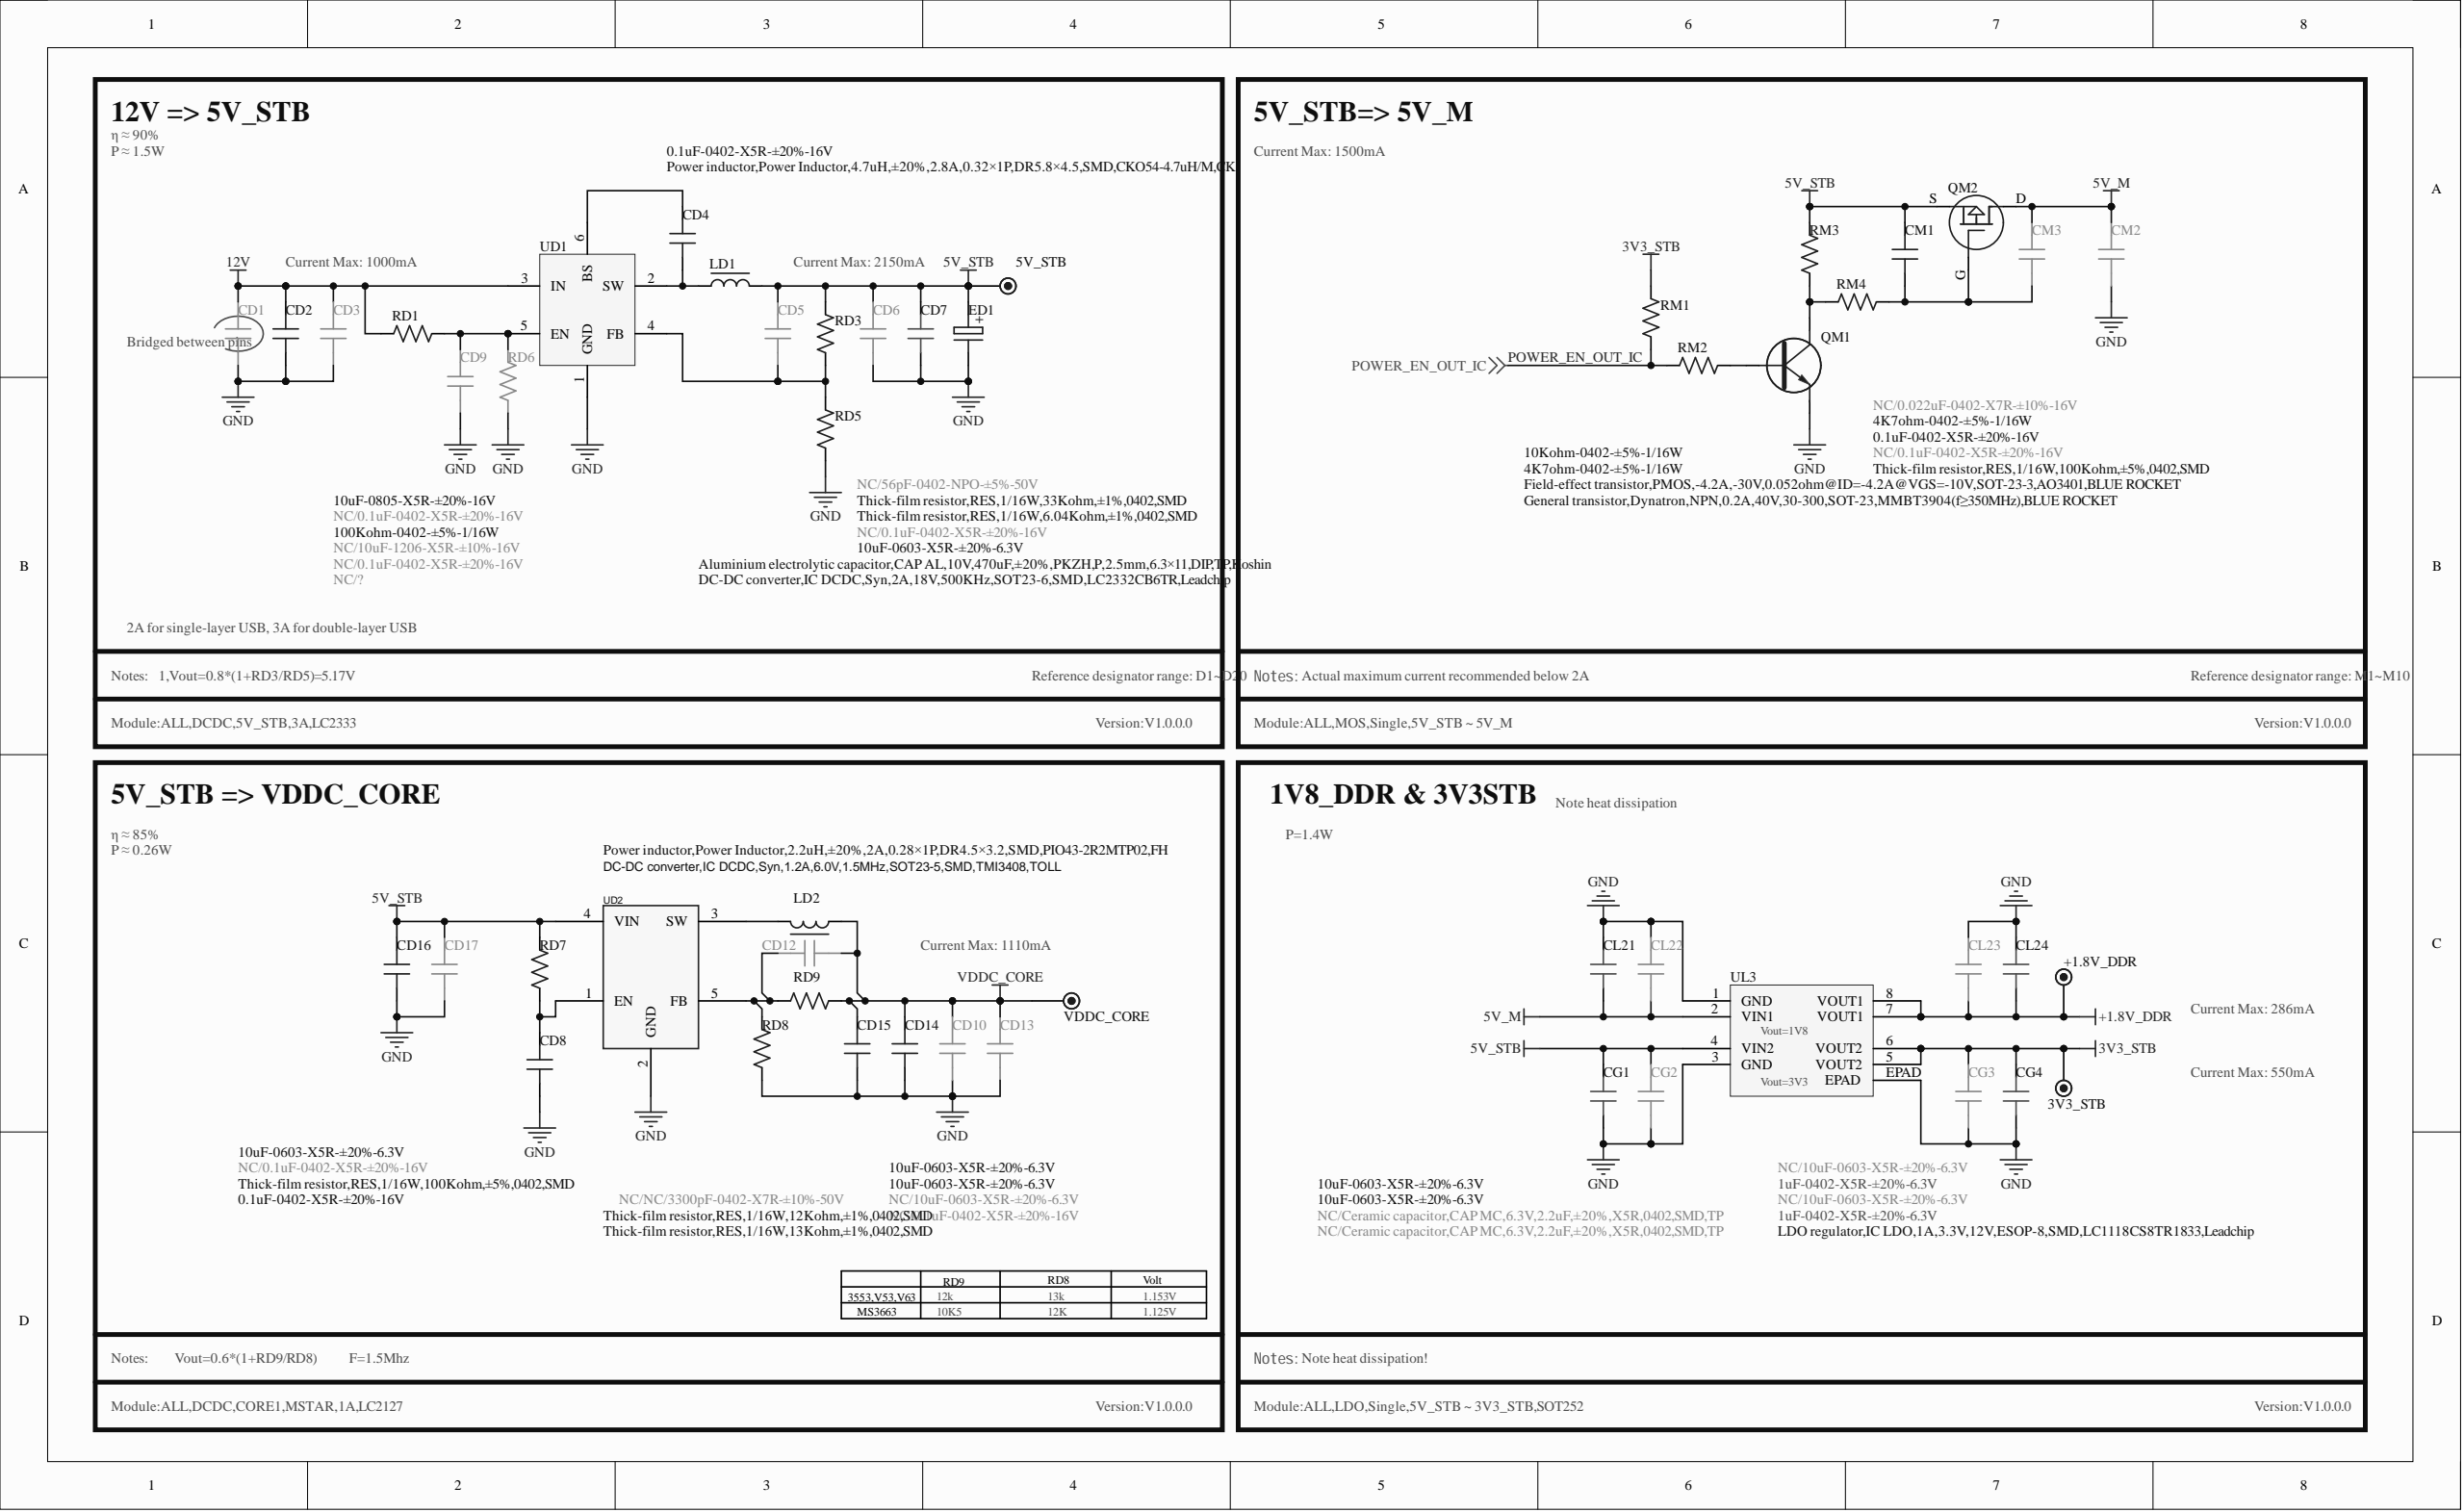Circuit board | Altium Designer | 578 parts | 300 nets | one sheet of the schematic
Parts on this sheet (reference | value | footprint):
CD1 | NC/10uF-1206-X5R-±10%-16V | C1206
CD2 | 10uF-0805-X5R-±20%-16V | C0805
CD3 | NC/0.1uF-0402-X5R-±20%-16V | C0402
CD4 | 0.1uF-0402-X5R-±20%-16V | C0402
CD5 | NC/56pF-0402-NPO-±5%-50V | C0402
CD6 | NC/0.1uF-0402-X5R-±20%-16V | C0402
CD7 | 10uF-0603-X5R-±20%-6.3V | C0603
CD8 | 0.1uF-0402-X5R-±20%-16V | C0402
CD9 | NC/0.1uF-0402-X5R-±20%-16V | C0402
CD10 | NC/10uF-0603-X5R-±20%-6.3V | C0603
CD12 | NC/NC/3300pF-0402-X7R-±10%-50V | C0402
CD13 | NC/0.1uF-0402-X5R-±20%-16V | C0402
CD14 | 10uF-0603-X5R-±20%-6.3V | C0603
CD15 | 10uF-0603-X5R-±20%-6.3V | C0603
CD16 | 10uF-0603-X5R-±20%-6.3V | C0603
CD17 | NC/0.1uF-0402-X5R-±20%-16V | C0402
CG1 | 10uF-0603-X5R-±20%-6.3V | C0603
CG2 | NC/Ceramic capacitor,CAP MC,6.3V,2.2uF,±20%,X5R,0402,SMD,TP | C0402
CG3 | NC/10uF-0603-X5R-±20%-6.3V | C0603
CG4 | 1uF-0402-X5R-±20%-6.3V | C0402
CL21 | 10uF-0603-X5R-±20%-6.3V | C0603
CL22 | NC/Ceramic capacitor,CAP MC,6.3V,2.2uF,±20%,X5R,0402,SMD,TP | C0402
CL23 | NC/10uF-0603-X5R-±20%-6.3V | C0603
CL24 | 1uF-0402-X5R-±20%-6.3V | C0402
CM1 | 0.1uF-0402-X5R-±20%-16V | C0402
CM2 | NC/0.1uF-0402-X5R-±20%-16V | C0402
CM3 | NC/0.022uF-0402-X7R-±10%-16V | C0402
LD1 | Power inductor,Power Inductor,4.7uH,±20%,2.8A,0.32×1P,DR5.8×4.5,SMD,CKO54-4.7uH/M,CK | L(5.8*4.5)-S
LD2 | Power inductor,Power Inductor,2.2uH,±20%,2A,0.28×1P,DR4.5×3.2,SMD,PIO43-2R2MTP02,FH | L(4.5*3.5)-S
QM1 | General transistor,Dynatron,NPN,0.2A,40V,30-300,SOT-23,MMBT3904(f=350MHz),BLUE ROCKET | SOT-23
QM2 | Field-effect transistor,PMOS,-4.2A,-30V,0.052ohm@ID=-4.2A@VGS=-10V,SOT-23-3,AO3401,BLUE ROCKET | SOT-23-1
RD1 | 100Kohm-0402-±5%-1/16W | R0402
RD3 | Thick-film resistor,RES,1/16W,33Kohm,±1%,0402,SMD | R0402
RD5 | Thick-film resistor,RES,1/16W,6.04Kohm,±1%,0402,SMD | R0402
RD6 | NC/? | R0402
RD7 | Thick-film resistor,RES,1/16W,100Kohm,±5%,0402,SMD | R0402
RD8 | Thick-film resistor,RES,1/16W,13Kohm,±1%,0402,SMD | R0402
RD9 | Thick-film resistor,RES,1/16W,12Kohm,±1%,0402,SMD | R0402
RM1 | 10Kohm-0402-±5%-1/16W | R0402
RM2 | 4K7ohm-0402-±5%-1/16W | R0402
RM3 | 4K7ohm-0402-±5%-1/16W | R0402
RM4 | Thick-film resistor,RES,1/16W,100Kohm,±5%,0402,SMD | R0402
UD1 | DC-DC converter,IC DCDC,Syn,2A,18V,500KHz,SOT23-6,SMD,LC2332CB6TR,Leadchip | SOT-23-6
UD2 | DC-DC converter,IC DCDC,Syn,1.2A,6.0V,1.5MHz,SOT23-5,SMD,TMI3408,TOLL | SOT-23-5
UL3 | LDO regulator,IC LDO,1A,3.3V,12V,ESOP-8,SMD,LC1118CS8TR1833,Leadchip | SOP8/1.27-3
Nets of these parts (net: part-pin ...):
VDDC_CORE: CD10-2 CD12-2 CD13-2 CD14-2 CD15-2 LD2-1 RD9-1
POWER_EN_OUT_IC: RM1-1 RM2-1
NetQM1_C: QM1-C RM3-1 RM4-1
NetQM1_B: QM1-B RM2-2
NetLD2_2: LD2-2 UD2-3
NetCM1_1: CM1-1 CM3-2 QM2-G RM4-2
NetCD12_1: CD12-1 RD8-1 RD9-2 UD2-5
NetCD9_2: CD9-2 RD1-2 RD6-2 UD1-5
NetCD8_2: CD8-2 RD7-1 UD2-1
NetCD5_1: CD5-1 RD3-1 RD5-2 UD1-4
NetCD4_2: CD4-2 UD1-6
NetCD4_1: CD4-1 LD1-1 UD1-2
GND: CD1-1 CD2-2 CD3-1 CD6-1 CD7-1 CD8-1 CD9-1 CD10-1 CD13-1 CD14-1 CD15-1 CD16-1 CD17-1 CG1-1 CG2-1 CG3-1 CG4-2 CL21-2 CL22-2 CL23-2 CL24-1 CM2-1 QM1-E RD5-1 RD6-1 RD8-2 UD1-1 UD2-2 UL3-1 UL3-3 UL3-EPAD
+1.8V_DDR: CL23-1 CL24-2 UL3-7 UL3-8
12V: CD1-2 CD2-1 CD3-2 RD1-1 UD1-3
5V_STB: CD5-2 CD6-2 CD7-2 CD16-2 CD17-2 CG1-2 CG2-2 CM1-2 LD1-2 QM2-S RD3-2 RD7-2 RM3-2 UD2-4 UL3-4
5V_M: CL21-1 CL22-1 CM2-2 CM3-1 QM2-D UL3-2
3V3_STB: CG3-2 CG4-1 RM1-2 UL3-5 UL3-6